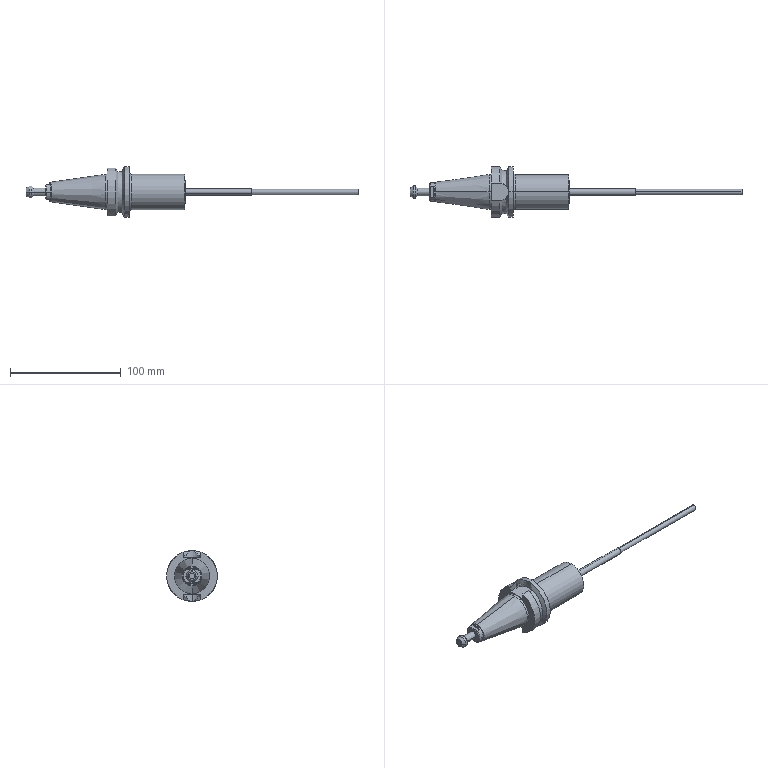Part | SolidWorks | 12 solids | 164 faces | box 300 x 46 x 46 mm | volume 105904 mm3 | plane 72 | cylinder 55 | cone 29 | torus 8 | commonest cylinder face diameters 3 x6 6 x6 21 x6 12 x4 46 x4 16.1 x3